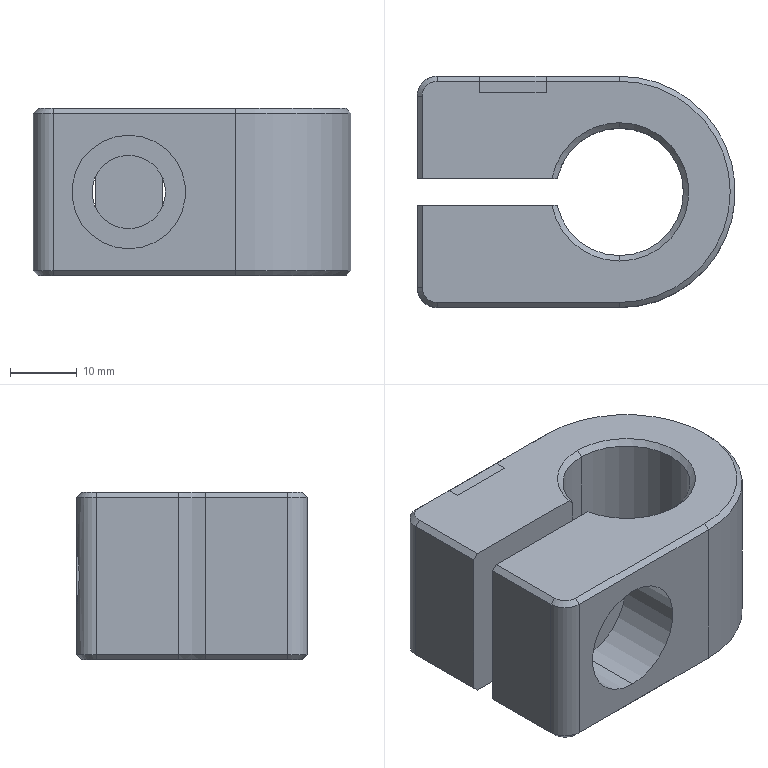Part | 2 solids | 70 faces | box 47.6 x 34.6 x 25 mm | volume 23828 mm3 | plane 36 | cylinder 17 | cone 16 | spline 1 | commonest cylinder face diameters 6 x4 11 x4 19.1 x3 25.1 x3 17 x2 34.6 x1